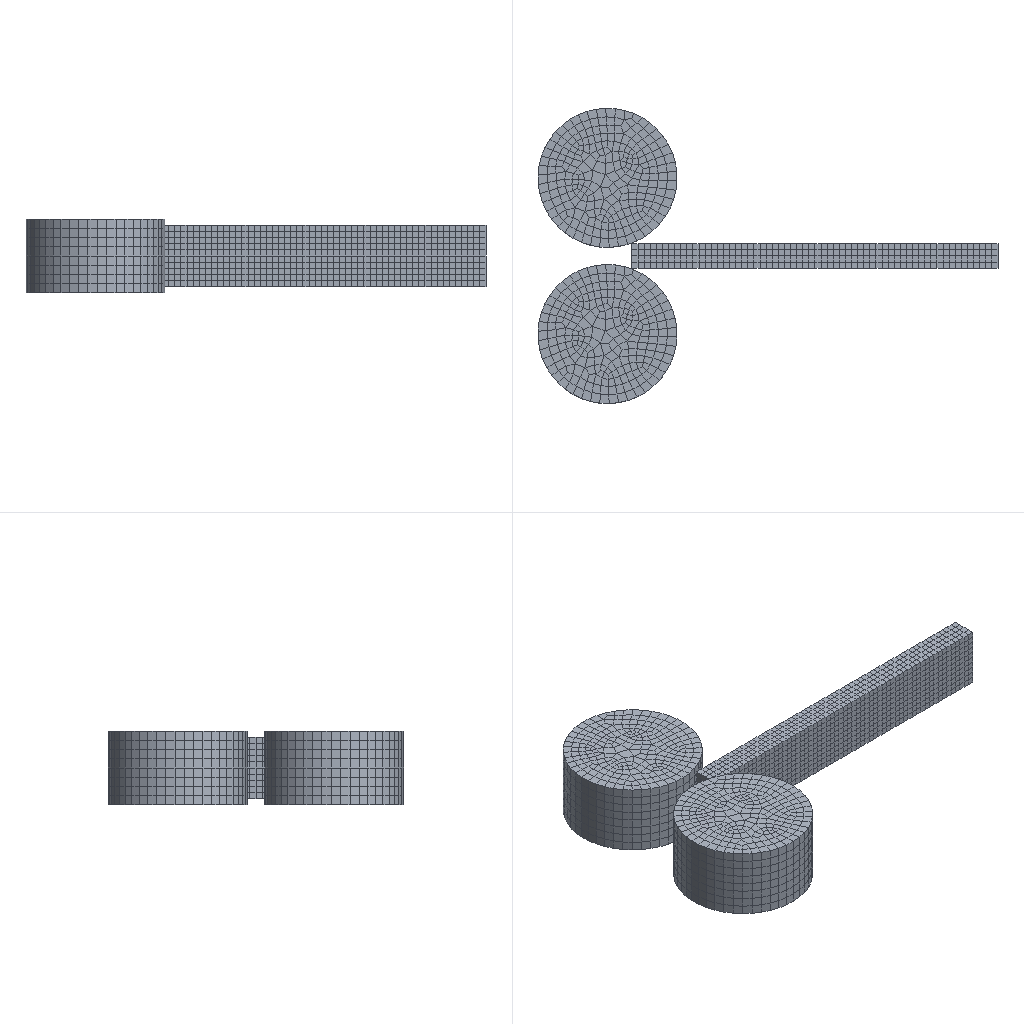Simulation study | abaqus
Set-up summary:
category,name,step,type,value,unit,region
solver,abaqus
solver,version,,,Abaqus/Explicit 2020
units,not stated in the deck,,not stated
analysis,deck,,dynamic temperature-displacement,dynamic temperature-displacement
load_step,Step-1,Step-1,dynamic temperature-displacement
load_step,requested,,,1
mesh,nodes,,,8397
mesh,elements,,,6496
element_type,C3D8R,,solid,4096
element_type,C3D8RT,,solid,2400
load,load commands in deck,,count,8
bc,support commands in deck,,count,22
material,GUN,,in results
material,WORK,,in results
check,setup vs results,,match,"per instance, exact: element labels, types and connectivity; labels of the nodes the elements use; coordinates of those nodes at SINGLE_PRECISION in 3 of 3 instance(s)"
Abaqus input file, long lists of numbers shortened:
*Heading
** Job name: Job-1 Model name: Model-1
** Generated by: Abaqus/CAE 2020
*Preprint, echo=NO, model=NO, history=NO, contact=NO
**
** PARTS
**
*Part, name=gun
*Node
      1,   541.986,  -176.498,           0.
      2,   560.971,  -101.054,           0.
** (2518 more lines like these left out)
*Element, type=C3D8R
   1,  495,  380,  324,  304,  215,  100,   44,   24
   2,  349,  350,  323,  303,   69,   70,   43,   23
** (2046 more lines like these left out)
*Node
   2521,           0., -3.4902433e-14,         600.
*Nset, nset=gun-RefPt_, internal
2521,
*Nset, nset=Set-1, generate
    1,  2520,     1
*Elset, elset=Set-1, generate
    1,  2048,     1
** Section: gun
*Solid Section, elset=Set-1, material=gun
,
*End Part
**
*Part, name=work
*Node
      1,           0.,        -200.,         500.
      2,           0.,        -150.,         500.
** (3353 more lines like these left out)
*Element, type=C3D8RT
   1,   56,   57,   62,   61,    1,    2,    7,    6
   2,   57,   58,   63,   62,    2,    3,    8,    7
** (2398 more lines like these left out)
*Nset, nset=Set-2, generate
    1,  3355,     1
*Elset, elset=Set-2, generate
    1,  2400,     1
** Section: work
*Solid Section, elset=Set-2, material=work
,
*End Part
**
**
** ASSEMBLY
**
*Assembly, name=Assembly
**
*Instance, name=gun-1, part=gun
       -200.,         540.,         -50.
*End Instance
**
*Instance, name=work-1, part=work
*End Instance
**
*Instance, name=gun-2, part=gun
       -200.,        -740.,         -50.
*End Instance
**
*Nset, nset=Set-5, instance=work-1, generate
    1,  3355,     1
*Elset, elset=Set-5, instance=work-1, generate
    1,  2400,     1
*Nset, nset=Set-6, instance=gun-2
 2521,
*Nset, nset=Set-7, instance=gun-1
 2521,
*Nset, nset=Set-8, instance=work-1, generate
 3301,  3355,     1
*Elset, elset=Set-8, instance=work-1, generate
 2361,  2400,     1
*Nset, nset=b_Set-1, instance=gun-1, generate
    1,  2520,     1
*Elset, elset=b_Set-1, instance=gun-1, generate
    1,  2048,     1
*Nset, nset=b_Set-3, instance=gun-2, generate
    1,  2520,     1
*Elset, elset=b_Set-3, instance=gun-2, generate
    1,  2048,     1
*Nset, nset=_PickedSet9, internal, instance=gun-1
 2521,
*Nset, nset=_PickedSet11, internal, instance=gun-2
 2521,
*Elset, elset=_Surf-5_S1, internal, instance=work-1, generate
 2361,  2400,     1
*Elset, elset=_Surf-5_S6, internal, instance=work-1, generate
    1,  2397,     4
*Elset, elset=_Surf-5_S2, internal, instance=work-1, generate
  1,  40,   1
*Elset, elset=_Surf-5_S4, internal, instance=work-1, generate
    4,  2400,     4
*Elset, elset=_Surf-5_S3, internal, instance=work-1
    1,    2,    3,    4,   41,   42,   43,   44,   81,   82,   83,   84,  121,  122,  123,  124
  161,  162,  163,  164,  201,  202,  203,  204,  241,  242,  243,  244,  281,  282,  283,  284
** (13 more lines like these left out)
*Elset, elset=_Surf-5_S5, internal, instance=work-1
   37,   38,   39,   40,   77,   78,   79,   80,  117,  118,  119,  120,  157,  158,  159,  160
  197,  198,  199,  200,  237,  238,  239,  240,  277,  278,  279,  280,  317,  318,  319,  320
** (13 more lines like these left out)
*Surface, type=ELEMENT, name=Surf-5
_Surf-5_S1, S1
_Surf-5_S6, S6
_Surf-5_S2, S2
_Surf-5_S4, S4
_Surf-5_S3, S3
_Surf-5_S5, S5
*Elset, elset=_Surf-6_S1, internal, instance=work-1, generate
 2361,  2400,     1
*Elset, elset=_Surf-6_S6, internal, instance=work-1, generate
    1,  2397,     4
*Elset, elset=_Surf-6_S2, internal, instance=work-1, generate
  1,  40,   1
*Elset, elset=_Surf-6_S4, internal, instance=work-1, generate
    4,  2400,     4
*Elset, elset=_Surf-6_S3, internal, instance=work-1
    1,    2,    3,    4,   41,   42,   43,   44,   81,   82,   83,   84,  121,  122,  123,  124
  161,  162,  163,  164,  201,  202,  203,  204,  241,  242,  243,  244,  281,  282,  283,  284
** (13 more lines like these left out)
*Elset, elset=_Surf-6_S5, internal, instance=work-1
   37,   38,   39,   40,   77,   78,   79,   80,  117,  118,  119,  120,  157,  158,  159,  160
  197,  198,  199,  200,  237,  238,  239,  240,  277,  278,  279,  280,  317,  318,  319,  320
** (13 more lines like these left out)
*Surface, type=ELEMENT, name=Surf-6
_Surf-6_S1, S1
_Surf-6_S6, S6
_Surf-6_S2, S2
_Surf-6_S4, S4
_Surf-6_S3, S3
_Surf-6_S5, S5
*Elset, elset=_Surf-7_S4, internal, instance=work-1, generate
    4,  2400,     4
*Surface, type=ELEMENT, name=Surf-7
_Surf-7_S4, S4
*Elset, elset=_Surf-8_S6, internal, instance=work-1, generate
    1,  2397,     4
*Surface, type=ELEMENT, name=Surf-8
_Surf-8_S6, S6
*Elset, elset=_Surf-9_S4, internal, instance=work-1, generate
    4,  2400,     4
*Surface, type=ELEMENT, name=Surf-9
_Surf-9_S4, S4
*Elset, elset=_Surf-10_S6, internal, instance=work-1, generate
    1,  2397,     4
*Surface, type=ELEMENT, name=Surf-10
_Surf-10_S6, S6
*Elset, elset=_Surf-11_S1, internal, instance=work-1, generate
 2361,  2400,     1
*Elset, elset=_Surf-11_S6, internal, instance=work-1, generate
    1,  2397,     4
*Elset, elset=_Surf-11_S2, internal, instance=work-1, generate
  1,  40,   1
*Elset, elset=_Surf-11_S3, internal, instance=work-1
    1,    2,    3,    4,   41,   42,   43,   44,   81,   82,   83,   84,  121,  122,  123,  124
  161,  162,  163,  164,  201,  202,  203,  204,  241,  242,  243,  244,  281,  282,  283,  284
** (13 more lines like these left out)
*Elset, elset=_Surf-11_S5, internal, instance=work-1
   37,   38,   39,   40,   77,   78,   79,   80,  117,  118,  119,  120,  157,  158,  159,  160
  197,  198,  199,  200,  237,  238,  239,  240,  277,  278,  279,  280,  317,  318,  319,  320
** (13 more lines like these left out)
*Surface, type=ELEMENT, name=Surf-11
_Surf-11_S1, S1
_Surf-11_S6, S6
_Surf-11_S2, S2
_Surf-11_S3, S3
_Surf-11_S5, S5
*Elset, elset=_Surf-12_S1, internal, instance=work-1, generate
 2361,  2400,     1
*Elset, elset=_Surf-12_S6, internal, instance=work-1, generate
    1,  2397,     4
*Elset, elset=_Surf-12_S2, internal, instance=work-1, generate
  1,  40,   1
*Elset, elset=_Surf-12_S3, internal, instance=work-1
    1,    2,    3,    4,   41,   42,   43,   44,   81,   82,   83,   84,  121,  122,  123,  124
  161,  162,  163,  164,  201,  202,  203,  204,  241,  242,  243,  244,  281,  282,  283,  284
** (13 more lines like these left out)
*Elset, elset=_Surf-12_S5, internal, instance=work-1
   37,   38,   39,   40,   77,   78,   79,   80,  117,  118,  119,  120,  157,  158,  159,  160
  197,  198,  199,  200,  237,  238,  239,  240,  277,  278,  279,  280,  317,  318,  319,  320
** (13 more lines like these left out)
*Surface, type=ELEMENT, name=Surf-12
_Surf-12_S1, S1
_Surf-12_S6, S6
_Surf-12_S2, S2
_Surf-12_S3, S3
_Surf-12_S5, S5
*Elset, elset=_m_Surf-1_S5, internal, instance=gun-1
    1,    2,    7,    8,   15,   17,   19,   21,   22,   24,   31,   32,   33,   35,   53,   55
   60,   62,   64,   66,   72,  257,  258,  263,  264,  271,  273,  275,  277,  278,  280,  287
** (9 more lines like these left out)
*Elset, elset=_m_Surf-1_S3, internal, instance=gun-1
    3,    4,    6,   10,   11,   12,   14,   25,   28,   30,   34,   36,   37,   38,   39,   40
   41,   42,   43,   44,   46,   47,   51,   69,   90,  259,  260,  262,  266,  267,  268,  270
** (11 more lines like these left out)
*Surface, type=ELEMENT, name=m_Surf-1
_m_Surf-1_S5, S5
_m_Surf-1_S3, S3
*Elset, elset=_m_Surf-3_S5, internal, instance=gun-2
    1,    2,    7,    8,   15,   17,   19,   21,   22,   24,   31,   32,   33,   35,   53,   55
   60,   62,   64,   66,   72,  257,  258,  263,  264,  271,  273,  275,  277,  278,  280,  287
** (9 more lines like these left out)
*Elset, elset=_m_Surf-3_S3, internal, instance=gun-2
    3,    4,    6,   10,   11,   12,   14,   25,   28,   30,   34,   36,   37,   38,   39,   40
   41,   42,   43,   44,   46,   47,   51,   69,   90,  259,  260,  262,  266,  267,  268,  270
** (11 more lines like these left out)
*Surface, type=ELEMENT, name=m_Surf-3
_m_Surf-3_S5, S5
_m_Surf-3_S3, S3
*Elset, elset=_s_Surf-1_S1, internal, instance=work-1, generate
 2361,  2400,     1
*Elset, elset=_s_Surf-1_S2, internal, instance=work-1, generate
  1,  40,   1
*Elset, elset=_s_Surf-1_S4, internal, instance=work-1, generate
    4,  2400,     4
*Elset, elset=_s_Surf-1_S3, internal, instance=work-1
    1,    2,    3,    4,   41,   42,   43,   44,   81,   82,   83,   84,  121,  122,  123,  124
  161,  162,  163,  164,  201,  202,  203,  204,  241,  242,  243,  244,  281,  282,  283,  284
** (13 more lines like these left out)
*Elset, elset=_s_Surf-1_S5, internal, instance=work-1
   37,   38,   39,   40,   77,   78,   79,   80,  117,  118,  119,  120,  157,  158,  159,  160
  197,  198,  199,  200,  237,  238,  239,  240,  277,  278,  279,  280,  317,  318,  319,  320
** (13 more lines like these left out)
*Surface, type=ELEMENT, name=s_Surf-1
_s_Surf-1_S1, S1
_s_Surf-1_S2, S2
_s_Surf-1_S4, S4
_s_Surf-1_S3, S3
_s_Surf-1_S5, S5
*Elset, elset=_s_Surf-3_S1, internal, instance=work-1, generate
 2361,  2400,     1
*Elset, elset=_s_Surf-3_S6, internal, instance=work-1, generate
    1,  2397,     4
*Elset, elset=_s_Surf-3_S2, internal, instance=work-1, generate
  1,  40,   1
*Elset, elset=_s_Surf-3_S3, internal, instance=work-1
    1,    2,    3,    4,   41,   42,   43,   44,   81,   82,   83,   84,  121,  122,  123,  124
  161,  162,  163,  164,  201,  202,  203,  204,  241,  242,  243,  244,  281,  282,  283,  284
** (13 more lines like these left out)
*Elset, elset=_s_Surf-3_S5, internal, instance=work-1
   37,   38,   39,   40,   77,   78,   79,   80,  117,  118,  119,  120,  157,  158,  159,  160
  197,  198,  199,  200,  237,  238,  239,  240,  277,  278,  279,  280,  317,  318,  319,  320
** (13 more lines like these left out)
*Surface, type=ELEMENT, name=s_Surf-3
_s_Surf-3_S1, S1
_s_Surf-3_S6, S6
_s_Surf-3_S2, S2
_s_Surf-3_S3, S3
_s_Surf-3_S5, S5
** Constraint: Constraint-1
*Rigid Body, ref node=_PickedSet9, elset=b_Set-1, position=CENTER OF MASS
** Constraint: Constraint-2
*Rigid Body, ref node=_PickedSet11, elset=b_Set-3, position=CENTER OF MASS
*End Assembly
**
** MATERIALS
**
*Material, name=gun
*Density
 7.8e-09,
*Elastic
500000., 0.2
*Material, name=work
*Conductivity
48.,
*Density
 7.8e-09,
*Elastic
210000., 0.3
*Expansion
 1.1e-05,
*Plastic
345.,0.
*Specific Heat
 4.8e+08,
**
** INTERACTION PROPERTIES
**
*Surface Interaction, name=IntProp-1
*Friction
 0.3,
*Surface Behavior, pressure-overclosure=HARD
*Gap Heat Generation
0.9, 0.5
*Surface Interaction, name=IntProp-2
*Friction
 0.45,
*Surface Behavior, pressure-overclosure=HARD
*Gap Heat Generation
0.9, 0.5
**
** PHYSICAL CONSTANTS
**
*Physical Constants, absolute zero=-273., stefan boltzmann=5.67e-08
**
** PREDEFINED FIELDS
**
** Name: Predefined Field-1   Type: Temperature
*Initial Conditions, type=TEMPERATURE
Set-5, 1200.
** ----------------------------------------------------------------
**
** STEP: Step-1
**
*Step, name=Step-1, nlgeom=YES
*Dynamic Temperature-displacement, Explicit
, 0.7
*Bulk Viscosity
0.06, 1.2
** Mass Scaling: Semi-Automatic
**               Whole Model
*Fixed Mass Scaling, factor=500.
**
** BOUNDARY CONDITIONS
**
** Name: BC-1 Type: 速度/角速度
*Boundary, type=VELOCITY
Set-6, 1, 1, 3000.
Set-6, 2, 2
Set-6, 3, 3
Set-6, 4, 4
Set-6, 5, 5
Set-6, 6, 6, 8.
** Name: BC-2 Type: 速度/角速度
*Boundary, type=VELOCITY
Set-7, 1, 1, 3000.
Set-7, 2, 2
Set-7, 3, 3
Set-7, 4, 4
Set-7, 5, 5
Set-7, 6, 6, -7.
** Name: BC-3 Type: 位移/转角
*Boundary
Set-8, 1, 1
Set-8, 2, 2
Set-8, 3, 3
Set-8, 4, 4
Set-8, 5, 5
Set-8, 6, 6
**
** INTERACTIONS
**
** Interaction: Int-1
*Contact Pair, interaction=IntProp-1, mechanical constraint=KINEMATIC, cpset=Int-1
m_Surf-1, s_Surf-1
** Interaction: Int-2
*Contact Pair, interaction=IntProp-2, mechanical constraint=KINEMATIC, cpset=Int-2
m_Surf-3, s_Surf-3
** Interaction: Int-3
*Sradiate
Surf-9, R, 25., 0.35
** Interaction: Int-4
*Sfilm
Surf-7, F, 25., 0.005
** Interaction: Int-5
*Sfilm
Surf-12, F, 25., 0.01
** Interaction: Int-6
*Sradiate
Surf-11, R, 25., 0.45
**
** OUTPUT REQUESTS
**
*Restart, write, number interval=1, time marks=NO
**
** FIELD OUTPUT: F-Output-1
**
*Output, field, number interval=100
*Node Output
A, NT, RF, RFL, U, V
*Element Output, directions=YES
E, EVF, HFL, LE, MISES, PE, PEEQ, PEEQVAVG, PEVAVG, S, SVAVG, TEMP
*Contact Output
CDISP, CSTRESS
**
** HISTORY OUTPUT: H-Output-1
**
*Output, history, variable=PRESELECT
*End Step
Results summary:
result,step,Step-1,completed,increments=5941 time=0.7/0.7
result,analysis,,,"dynamic temperature-displacement, explict"
result,last_loadstep,,,1
result,primary field,,,"U, NT11"
result,reaction total,,FX,-13884548.77,model units
result,reaction total,,FY,4929412.172,model units
result,reaction total,,FZ,-32309.403,model units